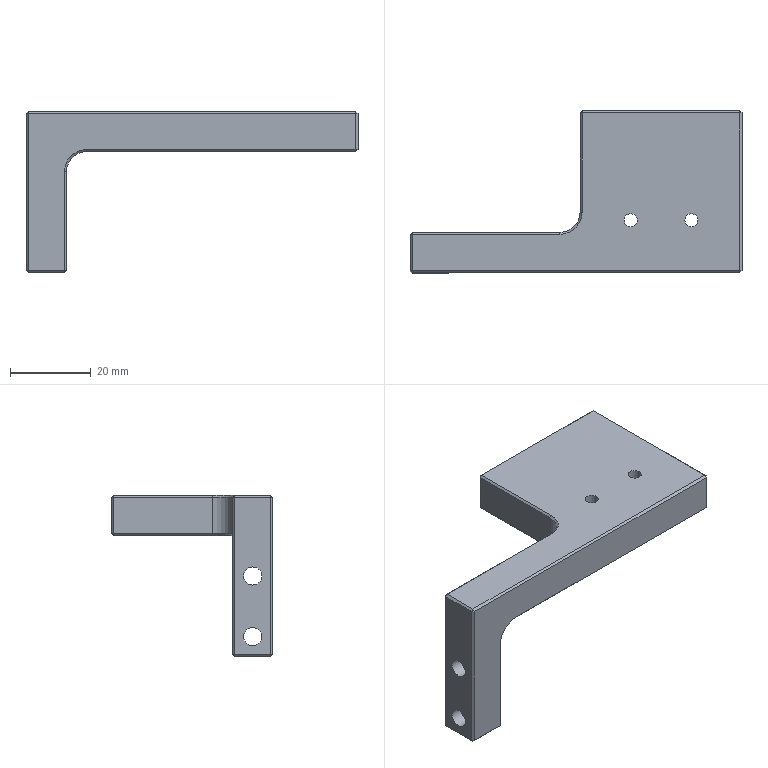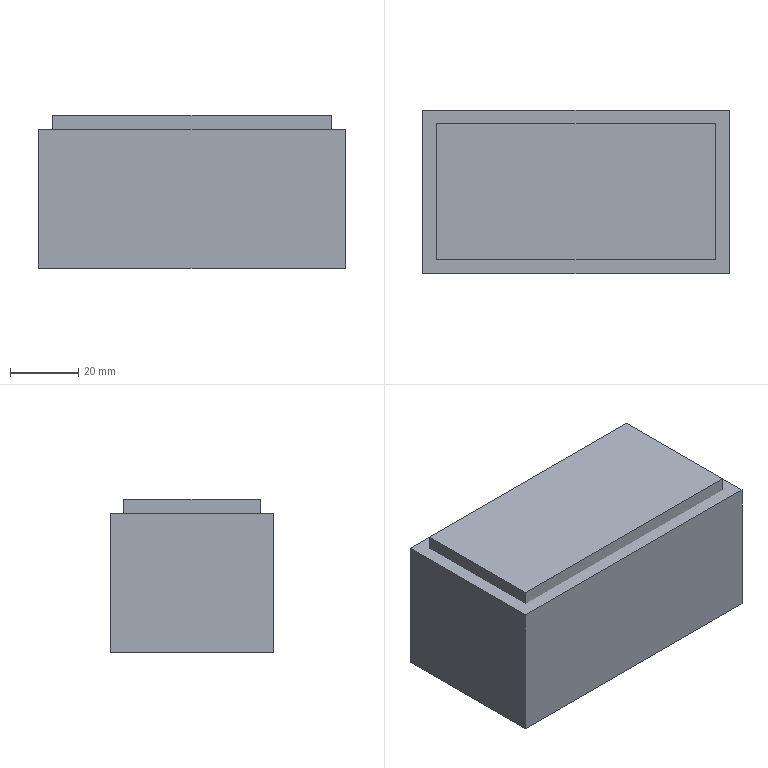CAM job | NX | 3+2 milling, drilling | part box 82 x 40 x 40 mm | stock box 90 x 48 x 45 mm
Tools:
number,name,description,diameter,corner_radius,flute_length,length,flutes
1,D63,Milling Tool-5 Parameters,63.0,0.0,50.0,75.0,2
9,D6A45,Milling Tool-5 Parameters,6.0,0.0,3.0,3.0,2
16,4.2ZT,Drilling Tool,3.2,0.0,35.0,50.0,2
2,D10,Milling Tool-5 Parameters,10.0,0.0,50.0,75.0,2
14,4.5ZT,Drilling Tool,4.5,0.0,35.0,50.0,2
Operations:
program,operation,operation_type,tool,method,geometry_group,spindle_rpm,surface_speed,feed_per_tooth,feed_cut,feed_plunge,cut_length_mm,path_length_mm,cut_time_min,machine_time_min
1-85-45-45毛胚,FLOOR_WALL,VolumeBased25DMillingOperation,D63,METHOD,A,6500.0,0.0,0.0,1250.0,100.0,165.0,219.0,0.132,0.1374
1-85-45-45毛胚,DRILLING,Operation,D6A45,METHOD,A,4000.0,75.0,0.0312,250.0,0.0,8.0,94.297,0.032,0.0406
1-85-45-45毛胚,DRILLING_COPY_1,Operation,4.2ZT,METHOD,A,2000.0,20.0,0.05,200.0,0.0,30.923,140.143,0.1546,0.1655
1-85-45-45毛胚,ADAPTIVE_MILLING,CavityMilling,D10,METHOD,A,7000.0,219.0,0.1429,2000.0,1000.0,10029.565,10305.264,5.018,5.045
1-85-45-45毛胚,ZLEVEL_PROFILE_COPY_COPY_1_COPY,ZLevelMilling,D10,METHOD,A,6500.0,326.0,0.0769,1000.0,1000.0,561.611,699.011,0.5616,0.5754
1-85-45-45毛胚,ZLEVEL_PROFILE_COPY_1_COPY_COPY_COPY_COPY_COPY,ZLevelMilling,D6A45,METHOD,A,7000.0,131.0,0.0714,1000.0,1000.0,258.322,488.54,0.2583,0.2813
2-85-45-45毛胚,DRILLING_COPY,Operation,D6A45,METHOD,B,4000.0,75.0,0.0312,250.0,0.0,8.0,94.297,0.032,0.0406
2-85-45-45毛胚,DRILLING_COPY_1_COPY,Operation,4.5ZT,METHOD,B,2000.0,20.0,0.05,200.0,0.0,31.704,141.705,0.1585,0.1695
3-85-45-45毛胚,FLOOR_WALL_COPY,VolumeBased25DMillingOperation,D63,METHOD,C,6500.0,0.0,0.0,1250.0,100.0,785.0,1639.001,0.628,0.7134
3-85-45-45毛胚,FLOOR_WALL_1,VolumeBased25DMillingOperation,D10,METHOD,C,7000.0,219.0,0.1786,2500.0,1000.0,7578.857,7837.999,3.039,3.065
3-85-45-45毛胚,FLOOR_WALL_1_COPY,VolumeBased25DMillingOperation,D10,METHOD,C,7000.0,219.0,0.1786,2500.0,1000.0,3674.426,3788.126,1.476,1.488
3-85-45-45毛胚,FLOOR_WALL_1_COPY_COPY_1_COPY,VolumeBased25DMillingOperation,D10,METHOD,C,7000.0,219.0,0.0714,1000.0,1000.0,751.455,1009.458,0.7515,0.7773
3-85-45-45毛胚,ZLEVEL_PROFILE_COPY_COPY_1_COPY_COPY,ZLevelMilling,D10,METHOD,C,6500.0,326.0,0.0769,1000.0,1000.0,57.05,178.362,0.057,0.0692
3-85-45-45毛胚,ZLEVEL_PROFILE_1,ZLevelMilling,D10,METHOD,C,7000.0,131.0,0.1786,2500.0,1000.0,3073.889,3185.939,1.232,1.243
3-85-45-45毛胚,ZLEVEL_PROFILE_COPY_1_COPY_COPY_COPY_COPY_COPY_COPY,ZLevelMilling,D6A45,METHOD,C,7000.0,131.0,0.0714,1000.0,1000.0,45.108,107.108,0.0451,0.0513
3-85-45-45毛胚,ZLEVEL_PROFILE_COPY_1_COPY_COPY_COPY_COPY_COPY_COPY_COPY,ZLevelMilling,D6A45,METHOD,C,7000.0,131.0,0.0714,1000.0,1000.0,219.045,640.314,0.219,0.2612